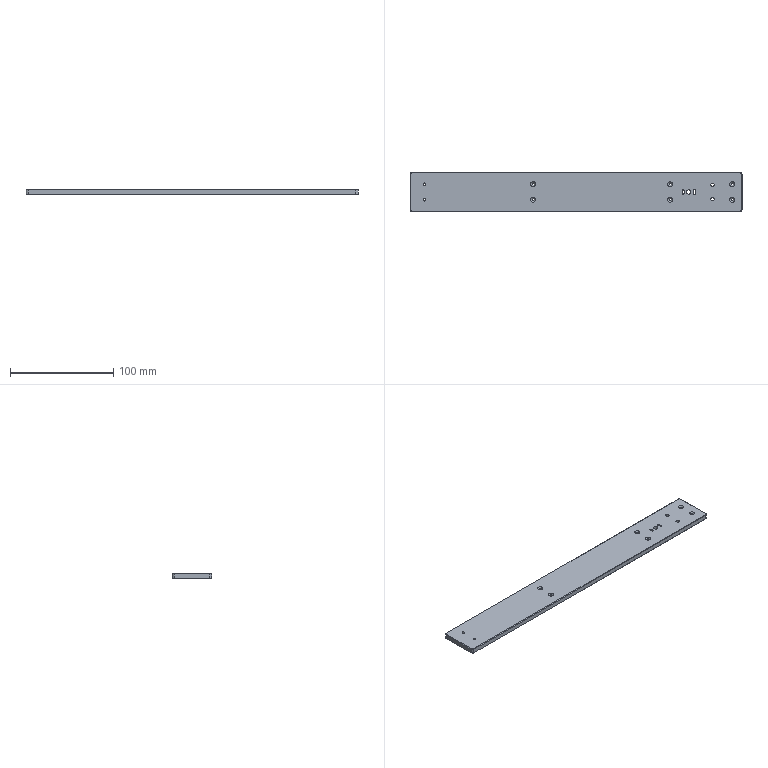Part | 1 solid | 59 faces | box 321 x 38 x 5 mm | volume 60333 mm3 | cylinder 23 | plane 22 | cone 14 | commonest cylinder face diameters 1 x8 2.459 x8 4 x4 3.242 x2 4.134 x1